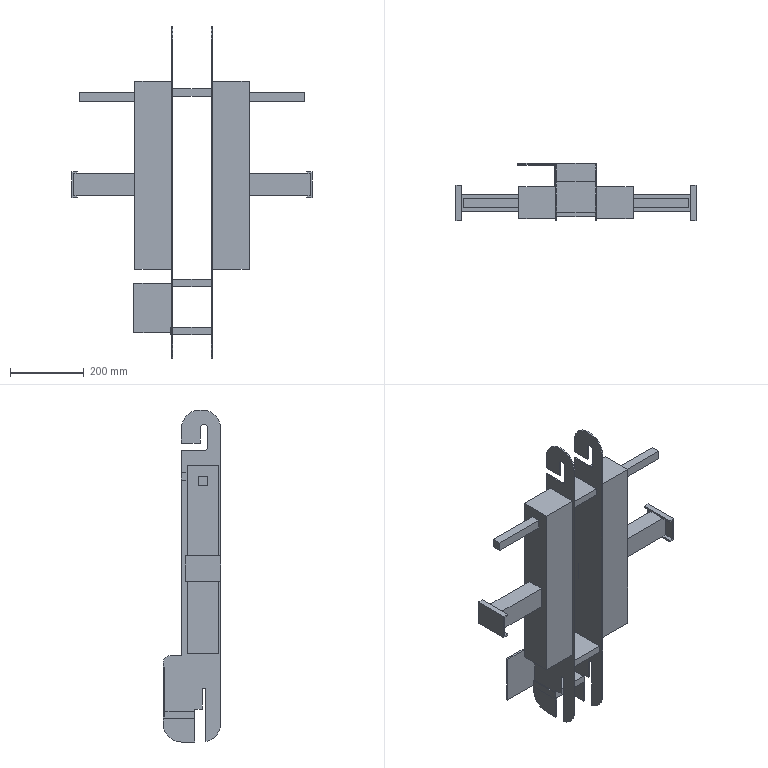Part | STEP file | 1 solid | 122 faces | box 651 x 157 x 900 mm | volume 11290183 mm3 | plane 106 | cylinder 16 | commonest cylinder face diameters 100 x8 20 x4 11.533 x2 40 x2